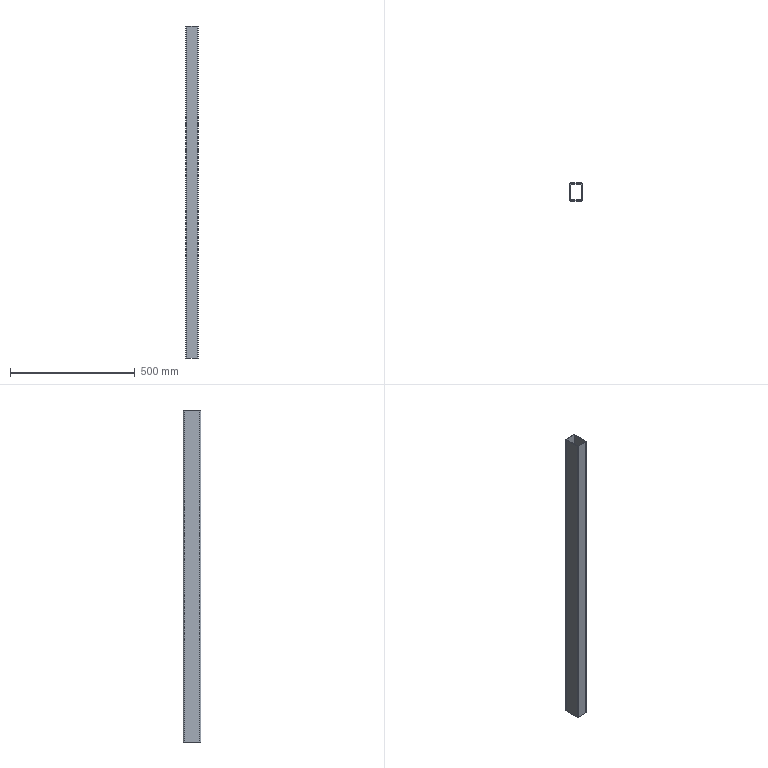Part | SolidWorks | features ExtruThin 1 | 1 solid | 18 faces | box 50 x 70 x 1330 mm | volume 892595 mm3 | plane 10 | cylinder 8 | commonest cylinder face diameters 2 x4 8 x4
STEP:
#1=CARTESIAN_POINT('',(-25.,-31.,1330.));
#2=VERTEX_POINT('',#1);
#3=CARTESIAN_POINT('',(-21.,-35.,1330.));
#4=VERTEX_POINT('',#3);
#5=CARTESIAN_POINT('',(-21.,-31.,1330.));
#6=DIRECTION('',(0.,0.,1.));
#7=DIRECTION('',(-1.,0.,0.));
#8=AXIS2_PLACEMENT_3D('',#5,#6,#7);
#9=CIRCLE('',#8,4.);
#10=EDGE_CURVE('',#2,#4,#9,.T.);
#11=ORIENTED_EDGE('',*,*,#10,.T.);
#12=CARTESIAN_POINT('',(21.,-35.,1330.));
#13=VERTEX_POINT('',#12);
#14=CARTESIAN_POINT('',(-21.,-35.,1330.));
#15=DIRECTION('',(1.,0.,0.));
#16=VECTOR('',#15,1000.);
#17=LINE('',#14,#16);
#18=EDGE_CURVE('',#4,#13,#17,.T.);
#19=ORIENTED_EDGE('',*,*,#18,.T.);
#20=CARTESIAN_POINT('',(25.,-31.,1330.));
#21=VERTEX_POINT('',#20);
#22=CARTESIAN_POINT('',(21.,-31.,1330.));
#23=DIRECTION('',(0.,0.,1.));
#24=DIRECTION('',(1.,0.,0.));
#25=AXIS2_PLACEMENT_3D('',#22,#23,#24);
#26=CIRCLE('',#25,4.);
#27=EDGE_CURVE('',#13,#21,#26,.T.);
#28=ORIENTED_EDGE('',*,*,#27,.T.);
#29=CARTESIAN_POINT('',(25.,31.,1330.));
#30=VERTEX_POINT('',#29);
#31=CARTESIAN_POINT('',(25.,-31.,1330.));
#32=DIRECTION('',(0.,1.,0.));
#33=VECTOR('',#32,1000.);
#34=LINE('',#31,#33);
#35=EDGE_CURVE('',#21,#30,#34,.T.);
#36=ORIENTED_EDGE('',*,*,#35,.T.);
#37=CARTESIAN_POINT('',(21.,35.,1330.));
#38=VERTEX_POINT('',#37);
#39=CARTESIAN_POINT('',(21.,31.,1330.));
#40=DIRECTION('',(0.,0.,1.));
#41=DIRECTION('',(-1.,0.,0.));
#42=AXIS2_PLACEMENT_3D('',#39,#40,#41);
#43=CIRCLE('',#42,4.);
#44=EDGE_CURVE('',#30,#38,#43,.T.);
#45=ORIENTED_EDGE('',*,*,#44,.T.);
#46=CARTESIAN_POINT('',(-21.,35.,1330.));
#47=VERTEX_POINT('',#46);
#48=CARTESIAN_POINT('',(-21.,35.,1330.));
#49=DIRECTION('',(-1.,0.,0.));
#50=VECTOR('',#49,1000.);
#51=LINE('',#48,#50);
#52=EDGE_CURVE('',#38,#47,#51,.T.);
#53=ORIENTED_EDGE('',*,*,#52,.T.);
#54=CARTESIAN_POINT('',(-25.,31.,1330.));
#55=VERTEX_POINT('',#54);
#56=CARTESIAN_POINT('',(-21.,31.,1330.));
#57=DIRECTION('',(0.,0.,1.));
#58=DIRECTION('',(-1.,0.,0.));
#59=AXIS2_PLACEMENT_3D('',#56,#57,#58);
#60=CIRCLE('',#59,4.);
#61=EDGE_CURVE('',#47,#55,#60,.T.);
#62=ORIENTED_EDGE('',*,*,#61,.T.);
#63=CARTESIAN_POINT('',(-25.,-31.,1330.));
#64=DIRECTION('',(0.,-1.,0.));
#65=VECTOR('',#64,1000.);
#66=LINE('',#63,#65);
#67=EDGE_CURVE('',#55,#2,#66,.T.);
#68=ORIENTED_EDGE('',*,*,#67,.T.);
#69=EDGE_LOOP('',(#11,#19,#28,#36,#45,#53,#62,#68));
#70=FACE_OUTER_BOUND('',#69,.T.);
#71=CARTESIAN_POINT('',(-21.,-32.,1330.));
#72=VERTEX_POINT('',#71);
#73=CARTESIAN_POINT('',(21.,-32.,1330.));
#74=VERTEX_POINT('',#73);
#75=CARTESIAN_POINT('',(-21.,-32.,1330.));
#76=DIRECTION('',(1.,0.,0.));
#77=VECTOR('',#76,1000.);
#78=LINE('',#75,#77);
#79=EDGE_CURVE('',#72,#74,#78,.T.);
#80=ORIENTED_EDGE('',*,*,#79,.F.);
#81=CARTESIAN_POINT('',(-22.,-31.,1330.));
#82=VERTEX_POINT('',#81);
#83=CARTESIAN_POINT('',(-21.,-31.,1330.));
#84=DIRECTION('',(0.,0.,1.));
#85=DIRECTION('',(-1.,0.,0.));
#86=AXIS2_PLACEMENT_3D('',#83,#84,#85);
#87=CIRCLE('',#86,1.);
#88=EDGE_CURVE('',#82,#72,#87,.T.);
#89=ORIENTED_EDGE('',*,*,#88,.F.);
#90=CARTESIAN_POINT('',(-22.,31.,1330.));
#91=VERTEX_POINT('',#90);
#92=CARTESIAN_POINT('',(-22.,-31.,1330.));
#93=DIRECTION('',(0.,-1.,0.));
#94=VECTOR('',#93,1000.);
#95=LINE('',#92,#94);
#96=EDGE_CURVE('',#91,#82,#95,.T.);
#97=ORIENTED_EDGE('',*,*,#96,.F.);
#98=CARTESIAN_POINT('',(-21.,32.,1330.));
#99=VERTEX_POINT('',#98);
#100=CARTESIAN_POINT('',(-21.,31.,1330.));
#101=DIRECTION('',(0.,0.,1.));
#102=DIRECTION('',(-1.,0.,0.));
#103=AXIS2_PLACEMENT_3D('',#100,#101,#102);
#104=CIRCLE('',#103,1.);
#105=EDGE_CURVE('',#99,#91,#104,.T.);
#106=ORIENTED_EDGE('',*,*,#105,.F.);
#107=CARTESIAN_POINT('',(21.,32.,1330.));
#108=VERTEX_POINT('',#107);
#109=CARTESIAN_POINT('',(-21.,32.,1330.));
#110=DIRECTION('',(-1.,0.,0.));
#111=VECTOR('',#110,1000.);
#112=LINE('',#109,#111);
#113=EDGE_CURVE('',#108,#99,#112,.T.);
#114=ORIENTED_EDGE('',*,*,#113,.F.);
#115=CARTESIAN_POINT('',(22.,31.,1330.));
#116=VERTEX_POINT('',#115);
#117=CARTESIAN_POINT('',(21.,31.,1330.));
#118=DIRECTION('',(0.,0.,1.));
#119=DIRECTION('',(-1.,0.,0.));
#120=AXIS2_PLACEMENT_3D('',#117,#118,#119);
#121=CIRCLE('',#120,1.);
#122=EDGE_CURVE('',#116,#108,#121,.T.);
#123=ORIENTED_EDGE('',*,*,#122,.F.);
#124=CARTESIAN_POINT('',(22.,-31.,1330.));
#125=VERTEX_POINT('',#124);
#126=CARTESIAN_POINT('',(22.,-31.,1330.));
#127=DIRECTION('',(0.,1.,0.));
#128=VECTOR('',#127,1000.);
#129=LINE('',#126,#128);
#130=EDGE_CURVE('',#125,#116,#129,.T.);
#131=ORIENTED_EDGE('',*,*,#130,.F.);
#132=CARTESIAN_POINT('',(21.,-31.,1330.));
#133=DIRECTION('',(0.,0.,1.));
#134=DIRECTION('',(-1.,0.,0.));
#135=AXIS2_PLACEMENT_3D('',#132,#133,#134);
#136=CIRCLE('',#135,1.);
#137=EDGE_CURVE('',#74,#125,#136,.T.);
#138=ORIENTED_EDGE('',*,*,#137,.F.);
#139=EDGE_LOOP('',(#80,#89,#97,#106,#114,#123,#131,#138));
#140=FACE_BOUND('',#139,.T.);
#141=CARTESIAN_POINT('',(-21.,-31.,1330.));
#142=DIRECTION('',(0.,0.,1.));
#143=DIRECTION('',(1.,0.,0.));
#144=AXIS2_PLACEMENT_3D('',#141,#142,#143);
#145=PLANE('',#144);
#146=ADVANCED_FACE('',(#70,#140),#145,.T.);
#147=CARTESIAN_POINT('',(-25.,-31.,0.));
#148=VERTEX_POINT('',#147);
#149=CARTESIAN_POINT('',(-21.,-35.,0.));
#150=VERTEX_POINT('',#149);
#151=CARTESIAN_POINT('',(-21.,-31.,0.));
#152=DIRECTION('',(0.,0.,1.));
#153=DIRECTION('',(-1.,0.,0.));
#154=AXIS2_PLACEMENT_3D('',#151,#152,#153);
#155=CIRCLE('',#154,4.);
#156=EDGE_CURVE('',#148,#150,#155,.T.);
#157=ORIENTED_EDGE('',*,*,#156,.F.);
#158=CARTESIAN_POINT('',(-25.,31.,0.));
#159=VERTEX_POINT('',#158);
#160=CARTESIAN_POINT('',(-25.,-31.,0.));
#161=DIRECTION('',(0.,-1.,0.));
#162=VECTOR('',#161,1000.);
#163=LINE('',#160,#162);
#164=EDGE_CURVE('',#159,#148,#163,.T.);
#165=ORIENTED_EDGE('',*,*,#164,.F.);
#166=CARTESIAN_POINT('',(-21.,35.,0.));
#167=VERTEX_POINT('',#166);
#168=CARTESIAN_POINT('',(-21.,31.,0.));
#169=DIRECTION('',(0.,0.,1.));
#170=DIRECTION('',(-1.,0.,0.));
#171=AXIS2_PLACEMENT_3D('',#168,#169,#170);
#172=CIRCLE('',#171,4.);
#173=EDGE_CURVE('',#167,#159,#172,.T.);
#174=ORIENTED_EDGE('',*,*,#173,.F.);
#175=CARTESIAN_POINT('',(21.,35.,0.));
#176=VERTEX_POINT('',#175);
#177=CARTESIAN_POINT('',(-21.,35.,0.));
#178=DIRECTION('',(-1.,0.,0.));
#179=VECTOR('',#178,1000.);
#180=LINE('',#177,#179);
#181=EDGE_CURVE('',#176,#167,#180,.T.);
#182=ORIENTED_EDGE('',*,*,#181,.F.);
#183=CARTESIAN_POINT('',(25.,31.,0.));
#184=VERTEX_POINT('',#183);
#185=CARTESIAN_POINT('',(21.,31.,0.));
#186=DIRECTION('',(0.,0.,1.));
#187=DIRECTION('',(-1.,0.,0.));
#188=AXIS2_PLACEMENT_3D('',#185,#186,#187);
#189=CIRCLE('',#188,4.);
#190=EDGE_CURVE('',#184,#176,#189,.T.);
#191=ORIENTED_EDGE('',*,*,#190,.F.);
#192=CARTESIAN_POINT('',(25.,-31.,0.));
#193=VERTEX_POINT('',#192);
#194=CARTESIAN_POINT('',(25.,-31.,0.));
#195=DIRECTION('',(0.,1.,0.));
#196=VECTOR('',#195,1000.);
#197=LINE('',#194,#196);
#198=EDGE_CURVE('',#193,#184,#197,.T.);
#199=ORIENTED_EDGE('',*,*,#198,.F.);
#200=CARTESIAN_POINT('',(21.,-35.,0.));
#201=VERTEX_POINT('',#200);
#202=CARTESIAN_POINT('',(21.,-31.,0.));
#203=DIRECTION('',(0.,0.,1.));
#204=DIRECTION('',(1.,0.,0.));
#205=AXIS2_PLACEMENT_3D('',#202,#203,#204);
#206=CIRCLE('',#205,4.);
#207=EDGE_CURVE('',#201,#193,#206,.T.);
#208=ORIENTED_EDGE('',*,*,#207,.F.);
#209=CARTESIAN_POINT('',(-21.,-35.,0.));
#210=DIRECTION('',(1.,0.,0.));
#211=VECTOR('',#210,1000.);
#212=LINE('',#209,#211);
#213=EDGE_CURVE('',#150,#201,#212,.T.);
#214=ORIENTED_EDGE('',*,*,#213,.F.);
#215=EDGE_LOOP('',(#157,#165,#174,#182,#191,#199,#208,#214));
#216=FACE_OUTER_BOUND('',#215,.T.);
#217=CARTESIAN_POINT('',(-22.,-31.,0.));
#218=VERTEX_POINT('',#217);
#219=CARTESIAN_POINT('',(-21.,-32.,0.));
#220=VERTEX_POINT('',#219);
#221=CARTESIAN_POINT('',(-21.,-31.,0.));
#222=DIRECTION('',(0.,0.,1.));
#223=DIRECTION('',(-1.,0.,0.));
#224=AXIS2_PLACEMENT_3D('',#221,#222,#223);
#225=CIRCLE('',#224,1.);
#226=EDGE_CURVE('',#218,#220,#225,.T.);
#227=ORIENTED_EDGE('',*,*,#226,.T.);
#228=CARTESIAN_POINT('',(21.,-32.,0.));
#229=VERTEX_POINT('',#228);
#230=CARTESIAN_POINT('',(-21.,-32.,0.));
#231=DIRECTION('',(1.,0.,0.));
#232=VECTOR('',#231,1000.);
#233=LINE('',#230,#232);
#234=EDGE_CURVE('',#220,#229,#233,.T.);
#235=ORIENTED_EDGE('',*,*,#234,.T.);
#236=CARTESIAN_POINT('',(22.,-31.,0.));
#237=VERTEX_POINT('',#236);
#238=CARTESIAN_POINT('',(21.,-31.,0.));
#239=DIRECTION('',(0.,0.,1.));
#240=DIRECTION('',(-1.,0.,0.));
#241=AXIS2_PLACEMENT_3D('',#238,#239,#240);
#242=CIRCLE('',#241,1.);
#243=EDGE_CURVE('',#229,#237,#242,.T.);
#244=ORIENTED_EDGE('',*,*,#243,.T.);
#245=CARTESIAN_POINT('',(22.,31.,0.));
#246=VERTEX_POINT('',#245);
#247=CARTESIAN_POINT('',(22.,-31.,0.));
#248=DIRECTION('',(0.,1.,0.));
#249=VECTOR('',#248,1000.);
#250=LINE('',#247,#249);
#251=EDGE_CURVE('',#237,#246,#250,.T.);
#252=ORIENTED_EDGE('',*,*,#251,.T.);
#253=CARTESIAN_POINT('',(21.,32.,0.));
#254=VERTEX_POINT('',#253);
#255=CARTESIAN_POINT('',(21.,31.,0.));
#256=DIRECTION('',(0.,0.,1.));
#257=DIRECTION('',(-1.,0.,0.));
#258=AXIS2_PLACEMENT_3D('',#255,#256,#257);
#259=CIRCLE('',#258,1.);
#260=EDGE_CURVE('',#246,#254,#259,.T.);
#261=ORIENTED_EDGE('',*,*,#260,.T.);
#262=CARTESIAN_POINT('',(-21.,32.,0.));
#263=VERTEX_POINT('',#262);
#264=CARTESIAN_POINT('',(-21.,32.,0.));
#265=DIRECTION('',(-1.,0.,0.));
#266=VECTOR('',#265,1000.);
#267=LINE('',#264,#266);
#268=EDGE_CURVE('',#254,#263,#267,.T.);
#269=ORIENTED_EDGE('',*,*,#268,.T.);
#270=CARTESIAN_POINT('',(-22.,31.,0.));
#271=VERTEX_POINT('',#270);
#272=CARTESIAN_POINT('',(-21.,31.,0.));
#273=DIRECTION('',(0.,0.,1.));
#274=DIRECTION('',(-1.,0.,0.));
#275=AXIS2_PLACEMENT_3D('',#272,#273,#274);
#276=CIRCLE('',#275,1.);
#277=EDGE_CURVE('',#263,#271,#276,.T.);
#278=ORIENTED_EDGE('',*,*,#277,.T.);
#279=CARTESIAN_POINT('',(-22.,-31.,0.));
#280=DIRECTION('',(0.,-1.,0.));
#281=VECTOR('',#280,1000.);
#282=LINE('',#279,#281);
#283=EDGE_CURVE('',#271,#218,#282,.T.);
#284=ORIENTED_EDGE('',*,*,#283,.T.);
#285=EDGE_LOOP('',(#227,#235,#244,#252,#261,#269,#278,#284));
#286=FACE_BOUND('',#285,.T.);
#287=CARTESIAN_POINT('',(-21.,-31.,0.));
#288=DIRECTION('',(0.,0.,1.));
#289=DIRECTION('',(1.,0.,0.));
#290=AXIS2_PLACEMENT_3D('',#287,#288,#289);
#291=PLANE('',#290);
#292=ADVANCED_FACE('',(#216,#286),#291,.F.);
#293=ORIENTED_EDGE('',*,*,#156,.T.);
#294=CARTESIAN_POINT('',(-21.,-35.,1330.));
#295=DIRECTION('',(0.,0.,-1.));
#296=VECTOR('',#295,1000.);
#297=LINE('',#294,#296);
#298=EDGE_CURVE('',#4,#150,#297,.T.);
#299=ORIENTED_EDGE('',*,*,#298,.F.);
#300=ORIENTED_EDGE('',*,*,#10,.F.);
#301=CARTESIAN_POINT('',(-25.,-31.,1330.));
#302=DIRECTION('',(0.,0.,-1.));
#303=VECTOR('',#302,1000.);
#304=LINE('',#301,#303);
#305=EDGE_CURVE('',#2,#148,#304,.T.);
#306=ORIENTED_EDGE('',*,*,#305,.T.);
#307=EDGE_LOOP('',(#293,#299,#300,#306));
#308=FACE_OUTER_BOUND('',#307,.T.);
#309=CARTESIAN_POINT('',(-21.,-31.,1330.));
#310=DIRECTION('',(0.,0.,-1.));
#311=DIRECTION('',(-1.,0.,0.));
#312=AXIS2_PLACEMENT_3D('',#309,#310,#311);
#313=CYLINDRICAL_SURFACE('',#312,4.);
#314=ADVANCED_FACE('',(#308),#313,.T.);
#315=ORIENTED_EDGE('',*,*,#213,.T.);
#316=CARTESIAN_POINT('',(21.,-35.,1330.));
#317=DIRECTION('',(0.,0.,-1.));
#318=VECTOR('',#317,1000.);
#319=LINE('',#316,#318);
#320=EDGE_CURVE('',#13,#201,#319,.T.);
#321=ORIENTED_EDGE('',*,*,#320,.F.);
#322=ORIENTED_EDGE('',*,*,#18,.F.);
#323=ORIENTED_EDGE('',*,*,#298,.T.);
#324=EDGE_LOOP('',(#315,#321,#322,#323));
#325=FACE_OUTER_BOUND('',#324,.T.);
#326=CARTESIAN_POINT('',(-21.,-35.,1330.));
#327=DIRECTION('',(0.,1.,0.));
#328=DIRECTION('',(0.,0.,1.));
#329=AXIS2_PLACEMENT_3D('',#326,#327,#328);
#330=PLANE('',#329);
#331=ADVANCED_FACE('',(#325),#330,.F.);
#332=ORIENTED_EDGE('',*,*,#207,.T.);
#333=CARTESIAN_POINT('',(25.,-31.,1330.));
#334=DIRECTION('',(0.,0.,-1.));
#335=VECTOR('',#334,1000.);
#336=LINE('',#333,#335);
#337=EDGE_CURVE('',#21,#193,#336,.T.);
#338=ORIENTED_EDGE('',*,*,#337,.F.);
#339=ORIENTED_EDGE('',*,*,#27,.F.);
#340=ORIENTED_EDGE('',*,*,#320,.T.);
#341=EDGE_LOOP('',(#332,#338,#339,#340));
#342=FACE_OUTER_BOUND('',#341,.T.);
#343=CARTESIAN_POINT('',(21.,-31.,1330.));
#344=DIRECTION('',(0.,0.,-1.));
#345=DIRECTION('',(-1.,0.,0.));
#346=AXIS2_PLACEMENT_3D('',#343,#344,#345);
#347=CYLINDRICAL_SURFACE('',#346,4.);
#348=ADVANCED_FACE('',(#342),#347,.T.);
#349=ORIENTED_EDGE('',*,*,#198,.T.);
#350=CARTESIAN_POINT('',(25.,31.,1330.));
#351=DIRECTION('',(0.,0.,-1.));
#352=VECTOR('',#351,1000.);
#353=LINE('',#350,#352);
#354=EDGE_CURVE('',#30,#184,#353,.T.);
#355=ORIENTED_EDGE('',*,*,#354,.F.);
#356=ORIENTED_EDGE('',*,*,#35,.F.);
#357=ORIENTED_EDGE('',*,*,#337,.T.);
#358=EDGE_LOOP('',(#349,#355,#356,#357));
#359=FACE_OUTER_BOUND('',#358,.T.);
#360=CARTESIAN_POINT('',(25.,-31.,1330.));
#361=DIRECTION('',(-1.,0.,0.));
#362=DIRECTION('',(0.,0.,1.));
#363=AXIS2_PLACEMENT_3D('',#360,#361,#362);
#364=PLANE('',#363);
#365=ADVANCED_FACE('',(#359),#364,.F.);
#366=ORIENTED_EDGE('',*,*,#190,.T.);
#367=CARTESIAN_POINT('',(21.,35.,1330.));
#368=DIRECTION('',(0.,0.,-1.));
#369=VECTOR('',#368,1000.);
#370=LINE('',#367,#369);
#371=EDGE_CURVE('',#38,#176,#370,.T.);
#372=ORIENTED_EDGE('',*,*,#371,.F.);
#373=ORIENTED_EDGE('',*,*,#44,.F.);
#374=ORIENTED_EDGE('',*,*,#354,.T.);
#375=EDGE_LOOP('',(#366,#372,#373,#374));
#376=FACE_OUTER_BOUND('',#375,.T.);
#377=CARTESIAN_POINT('',(21.,31.,1330.));
#378=DIRECTION('',(0.,0.,-1.));
#379=DIRECTION('',(-1.,0.,0.));
#380=AXIS2_PLACEMENT_3D('',#377,#378,#379);
#381=CYLINDRICAL_SURFACE('',#380,4.);
#382=ADVANCED_FACE('',(#376),#381,.T.);
#383=ORIENTED_EDGE('',*,*,#181,.T.);
#384=CARTESIAN_POINT('',(-21.,35.,1330.));
#385=DIRECTION('',(0.,0.,-1.));
#386=VECTOR('',#385,1000.);
#387=LINE('',#384,#386);
#388=EDGE_CURVE('',#47,#167,#387,.T.);
#389=ORIENTED_EDGE('',*,*,#388,.F.);
#390=ORIENTED_EDGE('',*,*,#52,.F.);
#391=ORIENTED_EDGE('',*,*,#371,.T.);
#392=EDGE_LOOP('',(#383,#389,#390,#391));
#393=FACE_OUTER_BOUND('',#392,.T.);
#394=CARTESIAN_POINT('',(-21.,35.,1330.));
#395=DIRECTION('',(0.,-1.,0.));
#396=DIRECTION('',(0.,0.,-1.));
#397=AXIS2_PLACEMENT_3D('',#394,#395,#396);
#398=PLANE('',#397);
#399=ADVANCED_FACE('',(#393),#398,.F.);
#400=ORIENTED_EDGE('',*,*,#173,.T.);
#401=CARTESIAN_POINT('',(-25.,31.,1330.));
#402=DIRECTION('',(0.,0.,-1.));
#403=VECTOR('',#402,1000.);
#404=LINE('',#401,#403);
#405=EDGE_CURVE('',#55,#159,#404,.T.);
#406=ORIENTED_EDGE('',*,*,#405,.F.);
#407=ORIENTED_EDGE('',*,*,#61,.F.);
#408=ORIENTED_EDGE('',*,*,#388,.T.);
#409=EDGE_LOOP('',(#400,#406,#407,#408));
#410=FACE_OUTER_BOUND('',#409,.T.);
#411=CARTESIAN_POINT('',(-21.,31.,1330.));
#412=DIRECTION('',(0.,0.,-1.));
#413=DIRECTION('',(-1.,0.,0.));
#414=AXIS2_PLACEMENT_3D('',#411,#412,#413);
#415=CYLINDRICAL_SURFACE('',#414,4.);
#416=ADVANCED_FACE('',(#410),#415,.T.);
#417=ORIENTED_EDGE('',*,*,#164,.T.);
#418=ORIENTED_EDGE('',*,*,#305,.F.);
#419=ORIENTED_EDGE('',*,*,#67,.F.);
#420=ORIENTED_EDGE('',*,*,#405,.T.);
#421=EDGE_LOOP('',(#417,#418,#419,#420));
#422=FACE_OUTER_BOUND('',#421,.T.);
#423=CARTESIAN_POINT('',(-25.,-31.,1330.));
#424=DIRECTION('',(1.,0.,0.));
#425=DIRECTION('',(0.,0.,-1.));
#426=AXIS2_PLACEMENT_3D('',#423,#424,#425);
#427=PLANE('',#426);
#428=ADVANCED_FACE('',(#422),#427,.F.);
#429=ORIENTED_EDGE('',*,*,#226,.F.);
#430=CARTESIAN_POINT('',(-22.,-31.,1330.));
#431=DIRECTION('',(0.,0.,-1.));
#432=VECTOR('',#431,1000.);
#433=LINE('',#430,#432);
#434=EDGE_CURVE('',#82,#218,#433,.T.);
#435=ORIENTED_EDGE('',*,*,#434,.F.);
#436=ORIENTED_EDGE('',*,*,#88,.T.);
#437=CARTESIAN_POINT('',(-21.,-32.,1330.));
#438=DIRECTION('',(0.,0.,-1.));
#439=VECTOR('',#438,1000.);
#440=LINE('',#437,#439);
#441=EDGE_CURVE('',#72,#220,#440,.T.);
#442=ORIENTED_EDGE('',*,*,#441,.T.);
#443=EDGE_LOOP('',(#429,#435,#436,#442));
#444=FACE_OUTER_BOUND('',#443,.T.);
#445=CARTESIAN_POINT('',(-21.,-31.,1330.));
#446=DIRECTION('',(0.,0.,-1.));
#447=DIRECTION('',(-1.,0.,0.));
#448=AXIS2_PLACEMENT_3D('',#445,#446,#447);
#449=CYLINDRICAL_SURFACE('',#448,1.);
#450=ADVANCED_FACE('',(#444),#449,.F.);
#451=ORIENTED_EDGE('',*,*,#234,.F.);
#452=ORIENTED_EDGE('',*,*,#441,.F.);
#453=ORIENTED_EDGE('',*,*,#79,.T.);
#454=CARTESIAN_POINT('',(21.,-32.,1330.));
#455=DIRECTION('',(0.,0.,-1.));
#456=VECTOR('',#455,1000.);
#457=LINE('',#454,#456);
#458=EDGE_CURVE('',#74,#229,#457,.T.);
#459=ORIENTED_EDGE('',*,*,#458,.T.);
#460=EDGE_LOOP('',(#451,#452,#453,#459));
#461=FACE_OUTER_BOUND('',#460,.T.);
#462=CARTESIAN_POINT('',(-21.,-32.,1330.));
#463=DIRECTION('',(0.,1.,0.));
#464=DIRECTION('',(0.,0.,1.));
#465=AXIS2_PLACEMENT_3D('',#462,#463,#464);
#466=PLANE('',#465);
#467=ADVANCED_FACE('',(#461),#466,.T.);
#468=ORIENTED_EDGE('',*,*,#243,.F.);
#469=ORIENTED_EDGE('',*,*,#458,.F.);
#470=ORIENTED_EDGE('',*,*,#137,.T.);
#471=CARTESIAN_POINT('',(22.,-31.,1330.));
#472=DIRECTION('',(0.,0.,-1.));
#473=VECTOR('',#472,1000.);
#474=LINE('',#471,#473);
#475=EDGE_CURVE('',#125,#237,#474,.T.);
#476=ORIENTED_EDGE('',*,*,#475,.T.);
#477=EDGE_LOOP('',(#468,#469,#470,#476));
#478=FACE_OUTER_BOUND('',#477,.T.);
#479=CARTESIAN_POINT('',(21.,-31.,1330.));
#480=DIRECTION('',(0.,0.,-1.));
#481=DIRECTION('',(-1.,0.,0.));
#482=AXIS2_PLACEMENT_3D('',#479,#480,#481);
#483=CYLINDRICAL_SURFACE('',#482,1.);
#484=ADVANCED_FACE('',(#478),#483,.F.);
#485=ORIENTED_EDGE('',*,*,#251,.F.);
#486=ORIENTED_EDGE('',*,*,#475,.F.);
#487=ORIENTED_EDGE('',*,*,#130,.T.);
#488=CARTESIAN_POINT('',(22.,31.,1330.));
#489=DIRECTION('',(0.,0.,-1.));
#490=VECTOR('',#489,1000.);
#491=LINE('',#488,#490);
#492=EDGE_CURVE('',#116,#246,#491,.T.);
#493=ORIENTED_EDGE('',*,*,#492,.T.);
#494=EDGE_LOOP('',(#485,#486,#487,#493));
#495=FACE_OUTER_BOUND('',#494,.T.);
#496=CARTESIAN_POINT('',(22.,-31.,1330.));
#497=DIRECTION('',(-1.,0.,0.));
#498=DIRECTION('',(0.,0.,1.));
#499=AXIS2_PLACEMENT_3D('',#496,#497,#498);
#500=PLANE('',#499);
#501=ADVANCED_FACE('',(#495),#500,.T.);
#502=ORIENTED_EDGE('',*,*,#260,.F.);
#503=ORIENTED_EDGE('',*,*,#492,.F.);
#504=ORIENTED_EDGE('',*,*,#122,.T.);
#505=CARTESIAN_POINT('',(21.,32.,1330.));
#506=DIRECTION('',(0.,0.,-1.));
#507=VECTOR('',#506,1000.);
#508=LINE('',#505,#507);
#509=EDGE_CURVE('',#108,#254,#508,.T.);
#510=ORIENTED_EDGE('',*,*,#509,.T.);
#511=EDGE_LOOP('',(#502,#503,#504,#510));
#512=FACE_OUTER_BOUND('',#511,.T.);
#513=CARTESIAN_POINT('',(21.,31.,1330.));
#514=DIRECTION('',(0.,0.,-1.));
#515=DIRECTION('',(-1.,0.,0.));
#516=AXIS2_PLACEMENT_3D('',#513,#514,#515);
#517=CYLINDRICAL_SURFACE('',#516,1.);
#518=ADVANCED_FACE('',(#512),#517,.F.);
#519=ORIENTED_EDGE('',*,*,#268,.F.);
#520=ORIENTED_EDGE('',*,*,#509,.F.);
#521=ORIENTED_EDGE('',*,*,#113,.T.);
#522=CARTESIAN_POINT('',(-21.,32.,1330.));
#523=DIRECTION('',(0.,0.,-1.));
#524=VECTOR('',#523,1000.);
#525=LINE('',#522,#524);
#526=EDGE_CURVE('',#99,#263,#525,.T.);
#527=ORIENTED_EDGE('',*,*,#526,.T.);
#528=EDGE_LOOP('',(#519,#520,#521,#527));
#529=FACE_OUTER_BOUND('',#528,.T.);
#530=CARTESIAN_POINT('',(-21.,32.,1330.));
#531=DIRECTION('',(0.,-1.,0.));
#532=DIRECTION('',(0.,0.,-1.));
#533=AXIS2_PLACEMENT_3D('',#530,#531,#532);
#534=PLANE('',#533);
#535=ADVANCED_FACE('',(#529),#534,.T.);
#536=ORIENTED_EDGE('',*,*,#277,.F.);
#537=ORIENTED_EDGE('',*,*,#526,.F.);
#538=ORIENTED_EDGE('',*,*,#105,.T.);
#539=CARTESIAN_POINT('',(-22.,31.,1330.));
#540=DIRECTION('',(0.,0.,-1.));
#541=VECTOR('',#540,1000.);
#542=LINE('',#539,#541);
#543=EDGE_CURVE('',#91,#271,#542,.T.);
#544=ORIENTED_EDGE('',*,*,#543,.T.);
#545=EDGE_LOOP('',(#536,#537,#538,#544));
#546=FACE_OUTER_BOUND('',#545,.T.);
#547=CARTESIAN_POINT('',(-21.,31.,1330.));
#548=DIRECTION('',(0.,0.,-1.));
#549=DIRECTION('',(-1.,0.,0.));
#550=AXIS2_PLACEMENT_3D('',#547,#548,#549);
#551=CYLINDRICAL_SURFACE('',#550,1.);
#552=ADVANCED_FACE('',(#546),#551,.F.);
#553=ORIENTED_EDGE('',*,*,#283,.F.);
#554=ORIENTED_EDGE('',*,*,#543,.F.);
#555=ORIENTED_EDGE('',*,*,#96,.T.);
#556=ORIENTED_EDGE('',*,*,#434,.T.);
#557=EDGE_LOOP('',(#553,#554,#555,#556));
#558=FACE_OUTER_BOUND('',#557,.T.);
#559=CARTESIAN_POINT('',(-22.,-31.,1330.));
#560=DIRECTION('',(1.,0.,0.));
#561=DIRECTION('',(0.,0.,-1.));
#562=AXIS2_PLACEMENT_3D('',#559,#560,#561);
#563=PLANE('',#562);
#564=ADVANCED_FACE('',(#558),#563,.T.);
#565=CLOSED_SHELL('',(#146,#292,#314,#331,#348,#365,#382,#399,#416,#428,#450,#467,#484,#501,#518,#535,#552,#564));
#566=MANIFOLD_SOLID_BREP('',#565);
#567=CARTESIAN_POINT('',(0.,0.,0.));
#568=DIRECTION('',(0.,0.,1.));
#569=DIRECTION('',(1.,0.,0.));
#570=AXIS2_PLACEMENT_3D('',#567,#568,#569);
#571=(LENGTH_UNIT()NAMED_UNIT(*)SI_UNIT(.MILLI.,.METRE.));
#572=UNCERTAINTY_MEASURE_WITH_UNIT(LENGTH_MEASURE(0.00001),#571,'','');
#573=(NAMED_UNIT(*)PLANE_ANGLE_UNIT()SI_UNIT($,.RADIAN.));
#574=(NAMED_UNIT(*)SI_UNIT($,.STERADIAN.)SOLID_ANGLE_UNIT());
#575=(GEOMETRIC_REPRESENTATION_CONTEXT(3)GLOBAL_UNCERTAINTY_ASSIGNED_CONTEXT((#572))GLOBAL_UNIT_ASSIGNED_CONTEXT((#571,#573,#574))REPRESENTATION_CONTEXT('',''));
#576=ADVANCED_BREP_SHAPE_REPRESENTATION('',(#566,#570),#575);